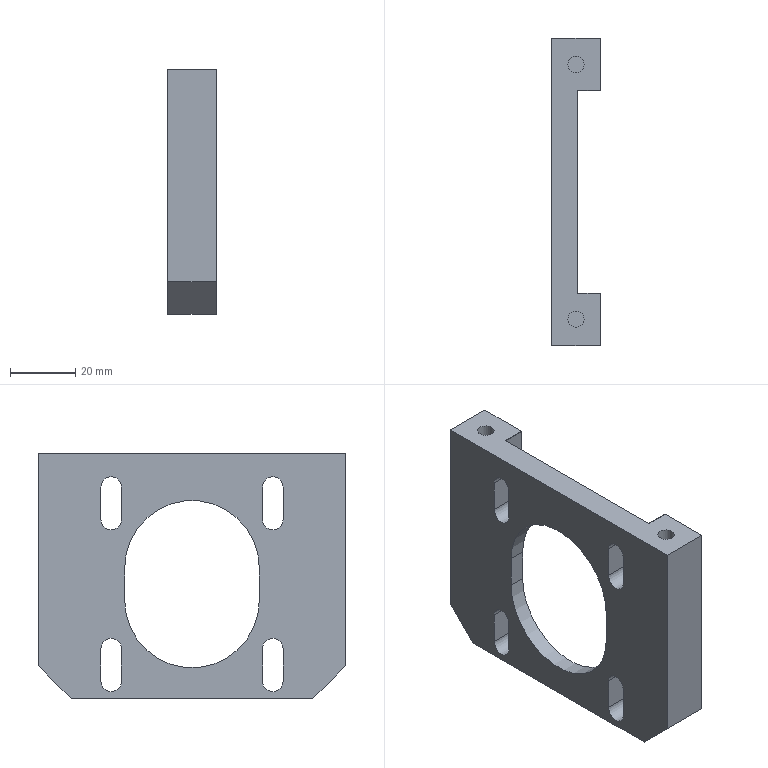CAM job | NX | 3+2 milling | part box 15 x 94 x 75 mm | stock box 20 x 99 x 80 mm
Tools:
number,name,description,diameter,corner_radius,flute_length,length,flutes
4,D4,平底铣刀-粗,4.0,0.0,25.0,75.0,2
9,D10,平底铣刀-粗,10.0,0.0,35.0,75.0,2
11,D4-J,平底铣刀-精,4.0,0.0,50.0,75.0,2
7,D6-J,平底铣刀-精,6.0,0.0,25.0,75.0,2
10,D10-J,平底铣刀-精,10.0,0.0,35.0,75.0,2
1,D80R0.8飞刀,圆鼻刀-粗,80.0,0.8,50.0,75.0,2
1,D80R0.8飞刀-J,圆鼻刀-精,80.0,0.8,50.0,75.0,2
2,D6倒角刀,倒角刀,6.0,0.0,3.0,25.0,2
Operations:
program,operation,operation_type,tool,method,geometry_group,spindle_rpm,surface_speed,feed_per_tooth,feed_cut,feed_plunge,cut_length_mm,path_length_mm,cut_time_min,machine_time_min
B,底壁铣飞面开粗_COPY,VolumeBased25DMillingOperation,D80R0.8飞刀,分层开粗-切深K-步距G,W-B,5000.0,1256.637,0.3,3000.0,100.0,3507.277,3757.881,1.169,1.194
B,底壁铣飞面精光_COPY,VolumeBased25DMillingOperation,D80R0.8飞刀-J,侧刃精光-切深K-步距G,W-B,5000.0,1256.637,0.1,1000.0,100.0,389.11,485.11,0.3891,0.3987
B,底壁铣分层开粗-中_COPY,VolumeBased25DMillingOperation,D10,分层开粗-切深K-步距G,W-B,8000.0,251.32,0.25,4000.0,100.0,9181.883,9464.699,2.296,2.324
B,底壁铣螺旋开粗-中_COPY,VolumeBased25DMillingOperation,D10,分层开粗-切深K-步距G,W-B,8000.0,251.327,0.125,2000.0,100.0,902.035,1016.935,0.451,0.4625
B,平面去毛刺6X45L_COPY,SurfaceContour,D6倒角刀,SURFACING_CHAMFER-DEPTH0-STEPG,W-B,6500.0,122.519,0.1154,1500.0,100.0,981.451,1845.932,0.6543,0.7407
B,底壁铣精光底面-中_COPY,VolumeBased25DMillingOperation,D10-J,精光步距切深关,W-B,8000.0,251.32,0.0625,1000.0,100.0,958.946,999.546,0.9589,0.963
B,底壁铣精光侧面-中-选底面_COPY,VolumeBased25DMillingOperation,D10-J,侧刃精光-切深K-步距G,W-B,8000.0,251.32,0.0625,1000.0,100.0,188.427,289.019,0.1884,0.1985
B,底壁铣精光侧面-中-选底面_COPY_1,VolumeBased25DMillingOperation,D10-J,侧刃精光-切深K-步距G,W-B,8000.0,251.32,0.0625,1000.0,100.0,168.89,216.49,0.1689,0.1736
A,顶面,FaceMilling,D80R0.8飞刀,侧刃精光-切深K-步距G,W-A,5000.0,1256.637,0.1,1000.0,100.0,188.0,224.0,0.188,0.1916
A,外形粗_2,VolumeBased25DMillingOperation,D10,METHOD,W-A,8000.0,251.327,0.3125,5000.0,80.0,7884.744,7938.744,1.577,1.582
A,型腔铣开粗-中_COPY,CavityMilling,D10,分层开粗-切深K-步距G,W-A,8000.0,251.327,0.1875,3000.0,100.0,4628.792,4955.586,1.543,1.591
A,通腰槽粗_1,VolumeBased25DMillingOperation,D4,METHOD,W-A,6000.0,75.398,0.1,1200.0,100.0,3942.576,4280.115,3.285,3.319
A,仅选体,SurfaceContour,D6倒角刀,METHOD,W-A,8000.0,150.796,0.1875,3000.0,100.0,657.088,1049.704,0.219,0.2583
A,框精_1,VolumeBased25DMillingOperation,D6-J,METHOD,W-A,6000.0,113.0,0.0833,1000.0,100.0,135.456,186.456,0.1355,0.1406
A,腰槽精_1,VolumeBased25DMillingOperation,D4-J,METHOD,W-A,6000.0,113.0,0.0417,500.0,100.0,235.632,650.797,0.4713,0.5128
A,外形半精_2,VolumeBased25DMillingOperation,D10-J,METHOD,W-A,8000.0,251.327,0.0625,1000.0,100.0,362.658,432.658,0.3627,0.3697